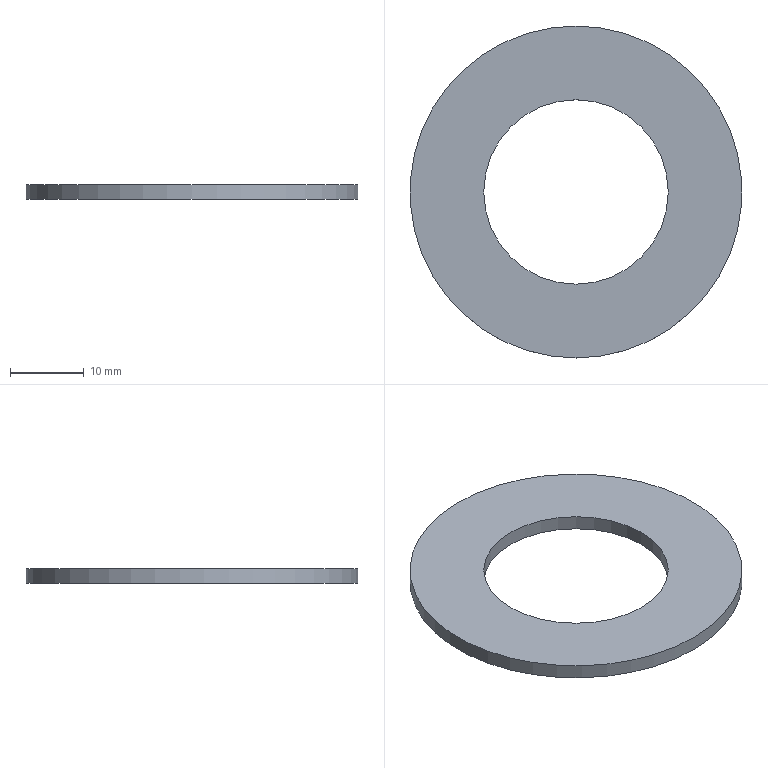Part | NX | features solid 2 | 1 solid | 4 faces | box 45 x 45 x 2 mm | volume 2199 mm3 | cylinder 2 | plane 2 | commonest cylinder face diameters 25 x1 45 x1
STEP:
#1=CARTESIAN_POINT('',(-652.5,-187.5,-53.));
#2=VERTEX_POINT('',#1);
#3=CARTESIAN_POINT('',(-652.5,-210.,-53.));
#4=DIRECTION('',(0.,0.,1.));
#5=DIRECTION('',(0.,1.,0.));
#6=AXIS2_PLACEMENT_3D('',#3,#4,#5);
#7=CIRCLE('',#6,22.5);
#8=EDGE_CURVE('',#2,#2,#7,.T.);
#9=ORIENTED_EDGE('',*,*,#8,.F.);
#10=EDGE_LOOP('',(#9));
#11=FACE_BOUND('',#10,.T.);
#12=CARTESIAN_POINT('',(-652.5,-187.5,-55.));
#13=VERTEX_POINT('',#12);
#14=CARTESIAN_POINT('',(-652.5,-210.,-55.));
#15=DIRECTION('',(0.,0.,1.));
#16=DIRECTION('',(0.,1.,0.));
#17=AXIS2_PLACEMENT_3D('',#14,#15,#16);
#18=CIRCLE('',#17,22.5);
#19=EDGE_CURVE('',#13,#13,#18,.T.);
#20=ORIENTED_EDGE('',*,*,#19,.T.);
#21=EDGE_LOOP('',(#20));
#22=FACE_BOUND('',#21,.T.);
#23=CARTESIAN_POINT('',(-652.5,-210.,-55.));
#24=DIRECTION('',(0.,0.,1.));
#25=DIRECTION('',(0.,1.,0.));
#26=AXIS2_PLACEMENT_3D('',#23,#24,#25);
#27=CYLINDRICAL_SURFACE('',#26,22.5);
#28=ADVANCED_FACE('',(#11,#22),#27,.T.);
#29=ORIENTED_EDGE('',*,*,#19,.F.);
#30=EDGE_LOOP('',(#29));
#31=FACE_BOUND('',#30,.T.);
#32=CARTESIAN_POINT('',(-652.5,-197.5,-55.));
#33=VERTEX_POINT('',#32);
#34=CARTESIAN_POINT('',(-652.5,-210.,-55.));
#35=DIRECTION('',(0.,0.,1.));
#36=DIRECTION('',(0.,1.,0.));
#37=AXIS2_PLACEMENT_3D('',#34,#35,#36);
#38=CIRCLE('',#37,12.5);
#39=EDGE_CURVE('',#33,#33,#38,.T.);
#40=ORIENTED_EDGE('',*,*,#39,.T.);
#41=EDGE_LOOP('',(#40));
#42=FACE_BOUND('',#41,.T.);
#43=CARTESIAN_POINT('',(-652.5,-210.,-55.));
#44=DIRECTION('',(0.,0.,-1.));
#45=DIRECTION('',(0.,-1.,0.));
#46=AXIS2_PLACEMENT_3D('',#43,#44,#45);
#47=PLANE('',#46);
#48=ADVANCED_FACE('',(#31,#42),#47,.T.);
#49=ORIENTED_EDGE('',*,*,#8,.T.);
#50=EDGE_LOOP('',(#49));
#51=FACE_BOUND('',#50,.T.);
#52=CARTESIAN_POINT('',(-652.5,-197.5,-53.));
#53=VERTEX_POINT('',#52);
#54=CARTESIAN_POINT('',(-652.5,-210.,-53.));
#55=DIRECTION('',(0.,0.,1.));
#56=DIRECTION('',(0.,1.,0.));
#57=AXIS2_PLACEMENT_3D('',#54,#55,#56);
#58=CIRCLE('',#57,12.5);
#59=EDGE_CURVE('',#53,#53,#58,.T.);
#60=ORIENTED_EDGE('',*,*,#59,.F.);
#61=EDGE_LOOP('',(#60));
#62=FACE_BOUND('',#61,.T.);
#63=CARTESIAN_POINT('',(-652.5,-210.,-53.));
#64=DIRECTION('',(0.,0.,-1.));
#65=DIRECTION('',(0.,-1.,0.));
#66=AXIS2_PLACEMENT_3D('',#63,#64,#65);
#67=PLANE('',#66);
#68=ADVANCED_FACE('',(#51,#62),#67,.F.);
#69=ORIENTED_EDGE('',*,*,#59,.T.);
#70=EDGE_LOOP('',(#69));
#71=FACE_BOUND('',#70,.T.);
#72=ORIENTED_EDGE('',*,*,#39,.F.);
#73=EDGE_LOOP('',(#72));
#74=FACE_BOUND('',#73,.T.);
#75=CARTESIAN_POINT('',(-652.5,-210.,-55.));
#76=DIRECTION('',(0.,0.,1.));
#77=DIRECTION('',(0.,1.,0.));
#78=AXIS2_PLACEMENT_3D('',#75,#76,#77);
#79=CYLINDRICAL_SURFACE('',#78,12.5);
#80=ADVANCED_FACE('',(#71,#74),#79,.F.);
#81=CLOSED_SHELL('',(#28,#48,#68,#80));
#82=MANIFOLD_SOLID_BREP('',#81);
#83=(LENGTH_UNIT()NAMED_UNIT(*)SI_UNIT(.MILLI.,.METRE.));
#84=UNCERTAINTY_MEASURE_WITH_UNIT(LENGTH_MEASURE(0.00001),#83,'','');
#85=(NAMED_UNIT(*)PLANE_ANGLE_UNIT()SI_UNIT($,.RADIAN.));
#86=(NAMED_UNIT(*)SI_UNIT($,.STERADIAN.)SOLID_ANGLE_UNIT());
#87=(GEOMETRIC_REPRESENTATION_CONTEXT(3)GLOBAL_UNCERTAINTY_ASSIGNED_CONTEXT((#84))GLOBAL_UNIT_ASSIGNED_CONTEXT((#83,#85,#86))REPRESENTATION_CONTEXT('',''));
#88=ADVANCED_BREP_SHAPE_REPRESENTATION('',(#82),#87);